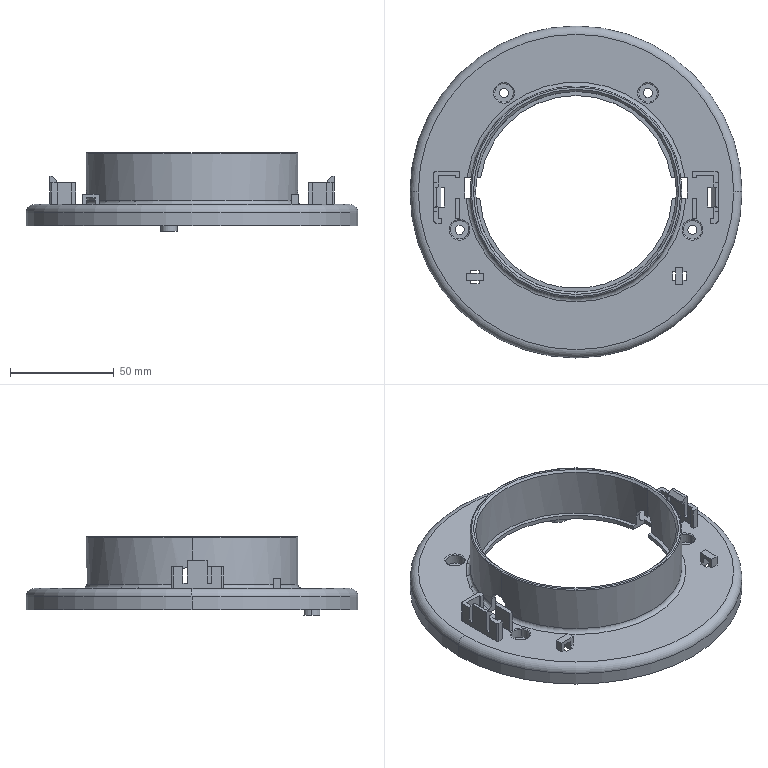Part | SolidWorks | features ICE 18, Fillet 7, Chamfer 2, CirPattern 2, Cut 1, Extrusion 1, MirrorPattern 1 | 1 solid | 198 faces | box 160 x 160 x 38 mm | volume 58176 mm3 | plane 112 | cylinder 68 | torus 16 | cone 2 | commonest cylinder face diameters 10 x14 6.3 x10 4.4 x8 9 x8 13 x8 2 x6